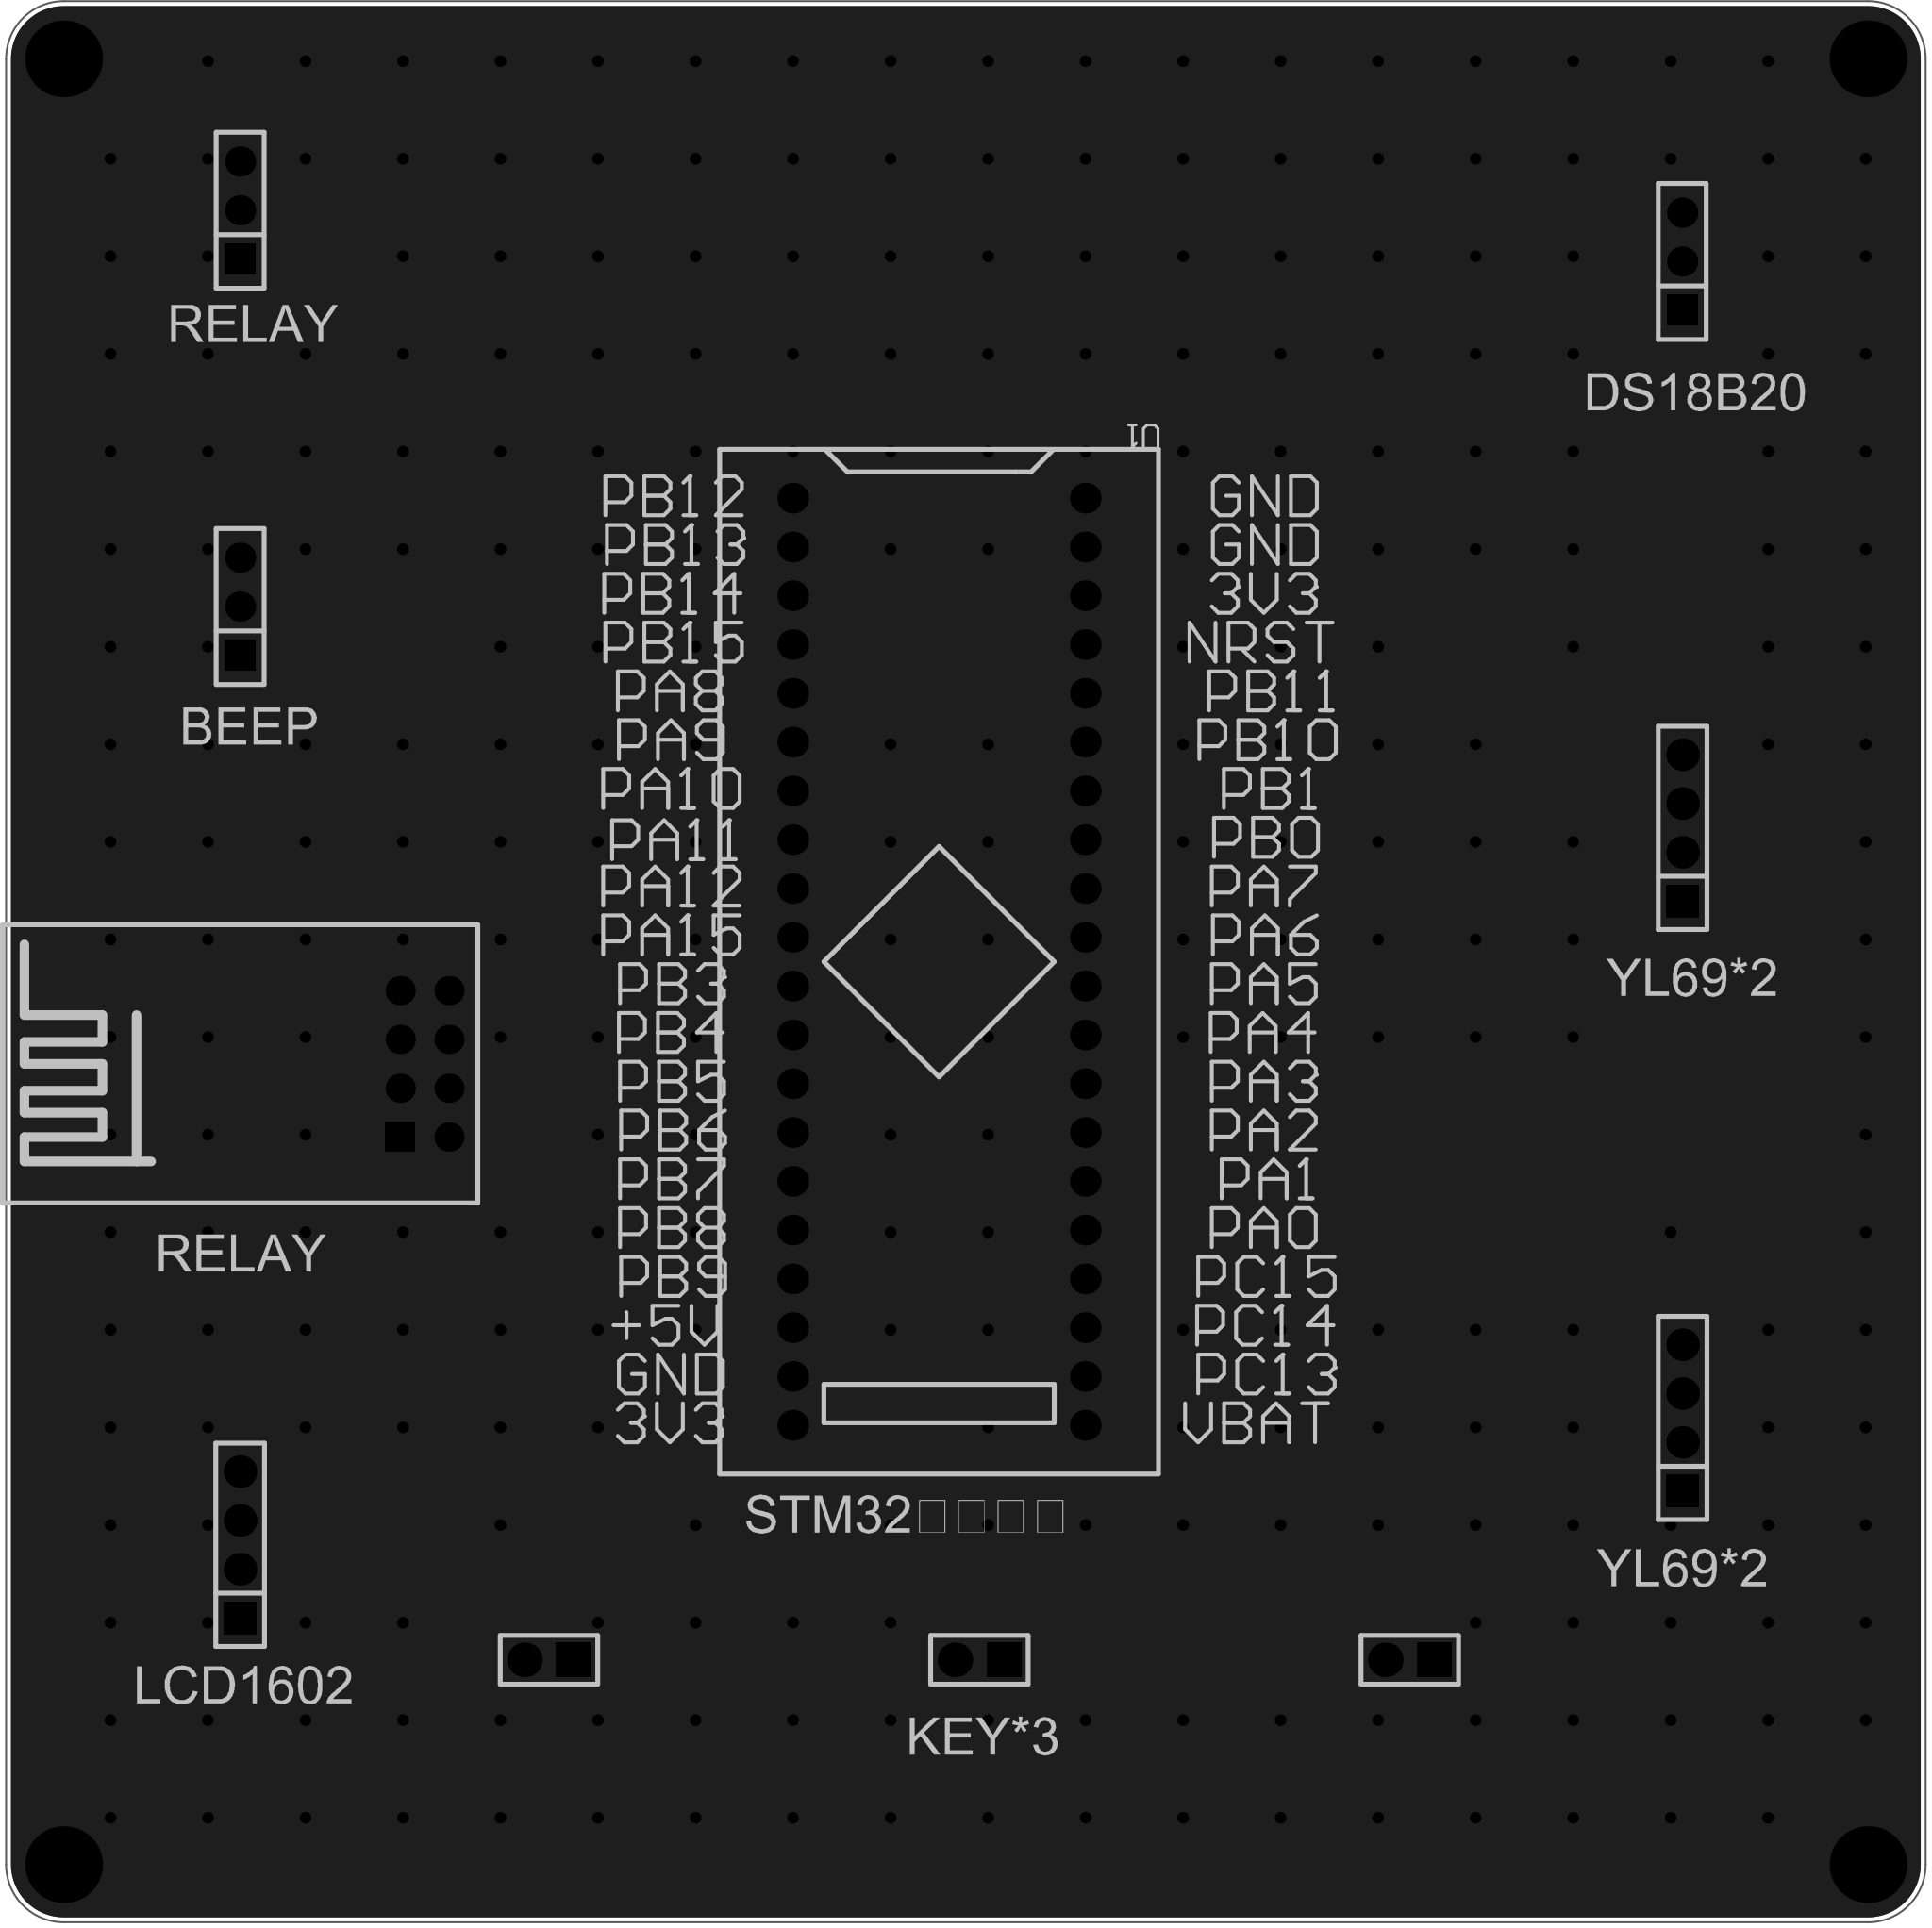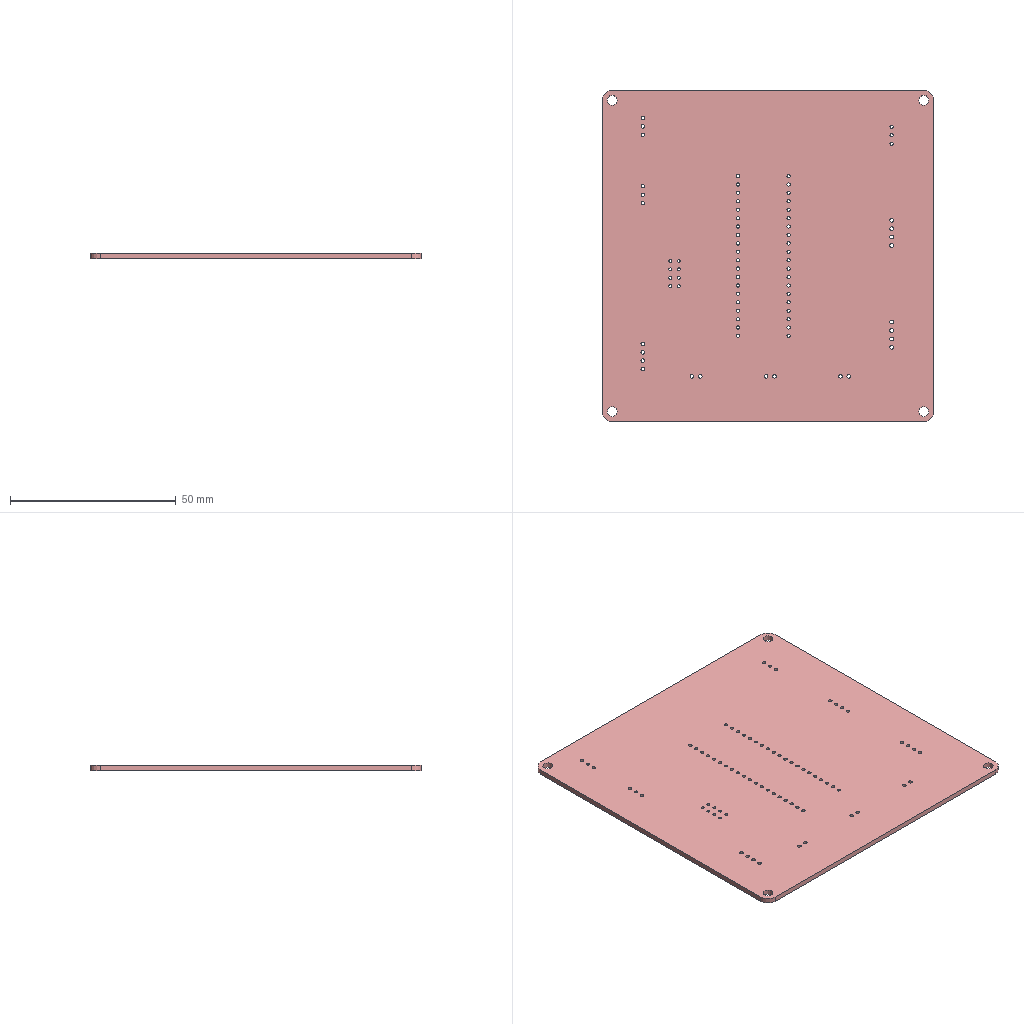Circuit board layout | Altium Designer | box 100 x 100 x 1.6 mm
Layer stack:
# Altium Designer layer stack of  (unit mm; dielectric type: 0 none, 1 core, 2 prepreg, 3 surface material)
index,name,kind,layer,copper_thickness_mm,dielectric_type,dielectric_thickness_mm,dielectric_material,dielectric_constant
0,Top Paste Mask Layer,other,,,,,,
1,Top Silkscreen Layer,other,,,,,,
2,Top Solder Mask Layer,dielectric,,,3,0.01,,3.3
3,Top Layer,copper,Top Layer,0.035,,,,
4,Dielectric1,dielectric,,,3,1.51,FR4,4.5
5,Bottom Layer,copper,Bottom Layer,0.035,,,,
6,Bottom Solder Mask Layer,dielectric,,,3,0.01,,3.3
7,Bottom Silkscreen Layer,other,,,,,,
8,Bottom Paste Mask Layer,other,,,,,,
# drill layer pairs: low layer,high layer
drill_pair,Top Layer,Bottom Layer
Part placement:
Designator,Comment,Layer,Footprint,Center-X(mm),Center-Y(mm),Rotation
U1,STM32F103C8T6-Card,TopLayer,CONN-TH_L53.3-W22.9_STM32F103C8T6-CARD,129.159,128.905,270
H1,,TopLayer,HDR-TH_2P-P2.54-V-M-1,153.681,92.566,180
H2,,TopLayer,HDR-TH_2P-P2.54-V-M-1,131.26,92.566,180
H3,,TopLayer,HDR-TH_2P-P2.54-V-M-1,108.839,92.566,180
H5,,TopLayer,HDR-TH_3P-P2.54-V-F,92.749,168.021,90
H8,,TopLayer,HDR-TH_4P-P2.54-V-F,167.894,105.156,90
H9,,TopLayer,HDR-TH_4P-P2.54-V-F,167.894,135.87,90
H10,,TopLayer,HDR-TH_4P-P2.54-V-F,92.749,98.552,90
H11,,TopLayer,HDR-TH_3P-P2.54-V-F,92.749,147.394,90
H12,,TopLayer,HDR-TH_3P-P2.54-V-F,167.874,165.354,90
U3,ESP8266-01S,TopLayer,WIFIM-TH_ESP8266-01S,102.362,123.588,90
Pad and via stacks:
# Altium Designer via and pad stacks of  (unit mm). Each distinct definition once, with the count of objects using it.
# via: kind,start_layer,end_layer,hole_mm,diameter_mm,mode(0 simple;1 top-mid-bottom;2 full stack),diameter_per_layer,count,example_net
# pad: kind,layer,hole_mm,hole_type(0 round;1 square;2 slot),plating,top_size,top_shape(1 round;2 rect;3 octagon;9 rounded rect),mid_size,bottom_size,mode,footprint,size_per_layer,count,example
pad,Multi-Layer,3,0,plated,4x4,1,4x4,4x4,0,,,4,1
pad,Multi-Layer,1,0,plated,1.6x1.6,1,1.6x1.6,1.6x1.6,0,CONN-TH_L53.3-W22.9_STM32F103C8T6-CARD,,40,U1.1
pad,Multi-Layer,1.1,0,plated,1.8x1.8,1,1.8x1.8,1.8x1.8,0,HDR-TH_2P-P2.54-V-M-1,,3,H1.2
pad,Multi-Layer,1.1,0,plated,1.8x1.8,2,1.8x1.8,1.8x1.8,0,HDR-TH_2P-P2.54-V-M-1,,3,H1.1
pad,Multi-Layer,1.02,0,plated,1.575x1.575,1,1.575x1.575,1.575x1.575,0,HDR-TH_3P-P2.54-V-F,,6,H5.3
pad,Multi-Layer,1.02,0,plated,1.575x1.575,2,1.575x1.575,1.575x1.575,0,HDR-TH_3P-P2.54-V-F,,3,H5.1
pad,Multi-Layer,1.1,0,plated,1.7x1.7,2,1.7x1.7,1.7x1.7,0,HDR-TH_4P-P2.54-V-F,,3,H8.1
pad,Multi-Layer,1.1,0,plated,1.7x1.7,1,1.7x1.7,1.7x1.7,0,HDR-TH_4P-P2.54-V-F,,9,H8.2
pad,Multi-Layer,0.9144,0,plated,1.524x1.524,1,1.524x1.524,1.524x1.524,0,WIFIM-TH_ESP8266-01S,,7,U3.8
pad,Multi-Layer,0.9144,0,plated,1.524x1.524,2,1.524x1.524,1.524x1.524,0,WIFIM-TH_ESP8266-01S,,1,U3.1
via,Top Layer,Bottom Layer,0.3048,0.61,0,,289,GND
Copper pours:
name,layer,net,type(0 solid;1 hatched;2 none)
Bottom Layer-GND,Bottom Layer,GND,0
Top Layer-GND,Top Layer,GND,0
Design rules, without the lines most boards share:
# Altium Designer design rules of  (exported by Altium Designer, unit mm)
# columns: name | kind | enabled | priority | scope1 | scope2 | descriptor | typed fields (field=value)
copperThickness1oz_2 | 2 | enabled | 2 | All | All | Width Constraint (Min=5mil) (Max=100mil) (Preferred=30mil) (All) |
viaSize | 11 | enabled | 1 | All | All | Routing Via (MinHoleWidth=11.811mil) (MaxHoleWidth=248.032mil) (PreferredHoleWidth=12.008mil) (MinWidth=19.685mil) (MaxWidth=393.701mil) (PreferedWidth=24.016mil) (All) | via_min_hole=0.3 via_max_hole=6.3 via_preferred_diameter=0.61 via_preferred_hole=0.305
solderMaskExpansion | 13 | enabled | 2 | All | All | Solder Mask Expansion (Expansion =2.008mil) (All) | expansion=0.051